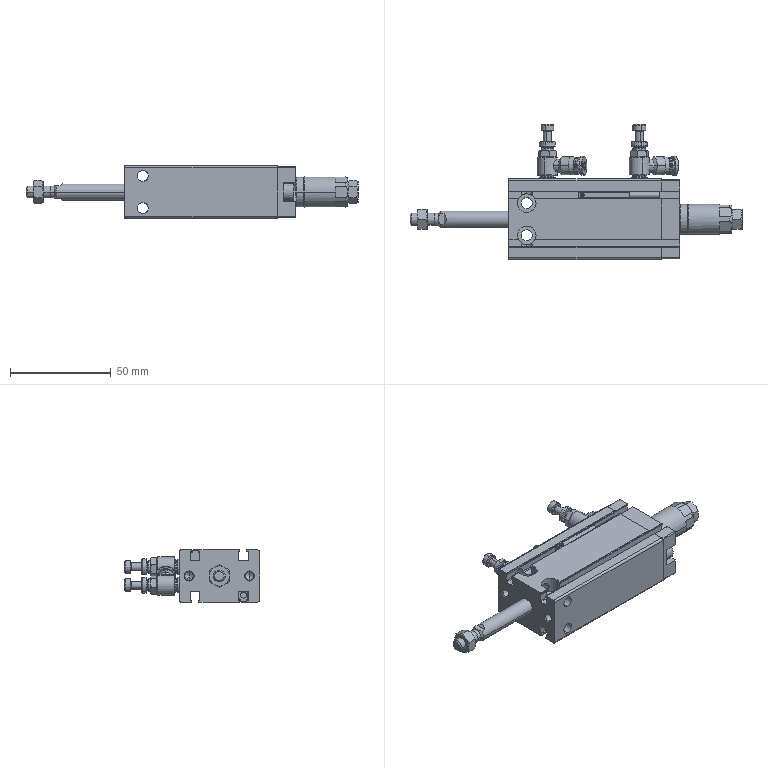Part | SolidWorks | features BaseBody 9, MoveFace 3 | 9 solids | 655 faces | box 165 x 67.1 x 26.6 mm | volume 85115 mm3 | plane 256 | cylinder 238 | cone 139 | spline 22 | commonest cylinder face diameters 0.4 x48 0.8 x16 5.5 x16 4 x12 8 x12 1 x10